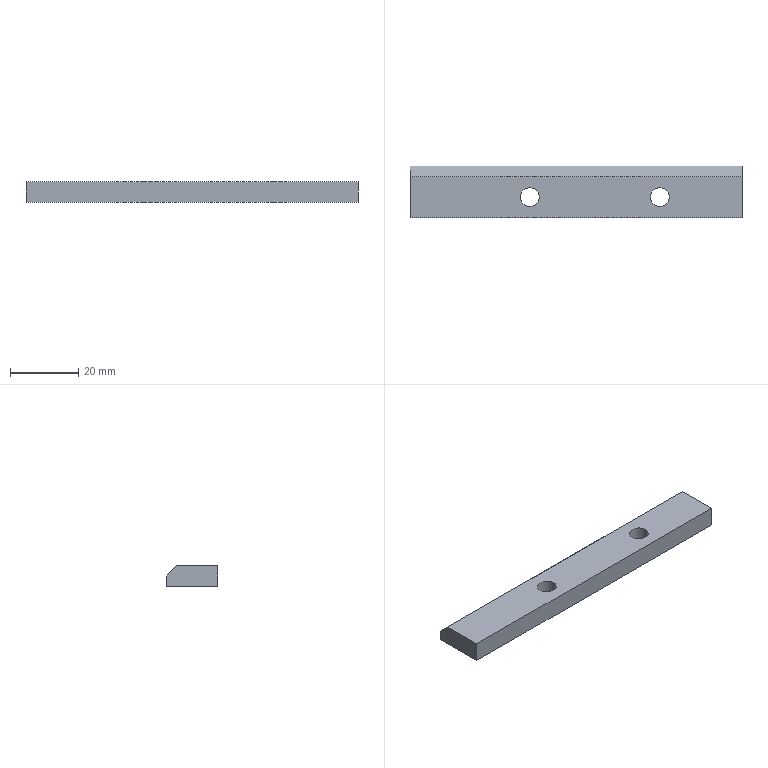Part | STEP file | cover plate 2 | 1 solid | 11 faces | box 97 x 15 x 6 mm | volume 8008 mm3 | plane 7 | cylinder 4 | commonest cylinder face diameters 5.5 x4
STEP:
#1=CARTESIAN_POINT('',(0.,0.,0.));
#2=DIRECTION('',(0.,0.,1.));
#3=DIRECTION('',(1.,0.,0.));
#4=AXIS2_PLACEMENT_3D('',#1,#2,#3);
#5=CARTESIAN_POINT('',(35.967,8.,0.));
#6=VERTEX_POINT('',#5);
#7=CARTESIAN_POINT('',(35.967,8.,6.));
#8=VERTEX_POINT('',#7);
#9=CARTESIAN_POINT('',(35.967,8.,6.));
#10=DIRECTION('',(0.,0.,1.));
#11=VECTOR('',#10,1.);
#12=LINE('',#9,#11);
#13=CARTESIAN_POINT('',(33.217,8.,6.));
#14=DIRECTION('',(0.,0.,1.));
#15=DIRECTION('',(1.,0.,0.));
#16=AXIS2_PLACEMENT_3D('',#13,#14,#15);
#17=CYLINDRICAL_SURFACE('',#16,2.75);
#18=CARTESIAN_POINT('',(6.283,0.));
#19=DIRECTION('',(0.,1.));
#20=VECTOR('',#19,1.);
#21=LINE('',#18,#20);
#22=(GEOMETRIC_REPRESENTATION_CONTEXT(2)PARAMETRIC_REPRESENTATION_CONTEXT()REPRESENTATION_CONTEXT('',''));
#23=DEFINITIONAL_REPRESENTATION('',(#21),#22);
#24=PCURVE('',#17,#23);
#25=CARTESIAN_POINT('',(33.217,8.,6.));
#26=DIRECTION('',(0.,0.,1.));
#27=DIRECTION('',(1.,0.,0.));
#28=AXIS2_PLACEMENT_3D('',#25,#26,#27);
#29=CYLINDRICAL_SURFACE('',#28,2.75);
#30=CARTESIAN_POINT('',(0.,0.));
#31=DIRECTION('',(0.,1.));
#32=VECTOR('',#31,1.);
#33=LINE('',#30,#32);
#34=(GEOMETRIC_REPRESENTATION_CONTEXT(2)PARAMETRIC_REPRESENTATION_CONTEXT()REPRESENTATION_CONTEXT('',''));
#35=DEFINITIONAL_REPRESENTATION('',(#33),#34);
#36=PCURVE('',#29,#35);
#37=SURFACE_CURVE('',#12,(#24,#36),.PCURVE_S1.);
#38=EDGE_CURVE('',#6,#8,#37,.T.);
#39=ORIENTED_EDGE('',*,*,#38,.T.);
#40=CARTESIAN_POINT('',(30.467,8.,6.));
#41=VERTEX_POINT('',#40);
#42=CARTESIAN_POINT('',(33.217,8.,6.));
#43=DIRECTION('',(0.,0.,1.));
#44=DIRECTION('',(1.,0.,0.));
#45=AXIS2_PLACEMENT_3D('',#42,#43,#44);
#46=CIRCLE('',#45,2.75);
#47=CARTESIAN_POINT('',(0.,0.));
#48=DIRECTION('',(1.,0.));
#49=VECTOR('',#48,1.);
#50=LINE('',#47,#49);
#51=(GEOMETRIC_REPRESENTATION_CONTEXT(2)PARAMETRIC_REPRESENTATION_CONTEXT()REPRESENTATION_CONTEXT('',''));
#52=DEFINITIONAL_REPRESENTATION('',(#50),#51);
#53=PCURVE('',#17,#52);
#54=CARTESIAN_POINT('',(40.217,2.,6.));
#55=DIRECTION('',(0.,0.,-1.));
#56=DIRECTION('',(-1.,0.,0.));
#57=AXIS2_PLACEMENT_3D('',#54,#55,#56);
#58=PLANE('',#57);
#59=CARTESIAN_POINT('',(4.25,6.));
#60=CARTESIAN_POINT('',(4.25,10.763));
#61=CARTESIAN_POINT('',(8.375,8.382));
#62=CARTESIAN_POINT('',(12.5,6.));
#63=CARTESIAN_POINT('',(8.375,3.618));
#64=CARTESIAN_POINT('',(4.25,1.237));
#65=CARTESIAN_POINT('',(4.25,6.));
#66=(BOUNDED_CURVE()B_SPLINE_CURVE(2,(#59,#60,#61,#62,#63,#64,#65),.UNSPECIFIED.,.T.,.F.)B_SPLINE_CURVE_WITH_KNOTS((1,2,2,2,2,1),(-2.094,0.,2.094,4.189,6.283,8.378),.UNSPECIFIED.)CURVE()GEOMETRIC_REPRESENTATION_ITEM()RATIONAL_B_SPLINE_CURVE((1.,0.5,1.,0.5,1.,0.5,1.))REPRESENTATION_ITEM(''));
#67=(GEOMETRIC_REPRESENTATION_CONTEXT(2)PARAMETRIC_REPRESENTATION_CONTEXT()REPRESENTATION_CONTEXT('',''));
#68=DEFINITIONAL_REPRESENTATION('',(#66),#67);
#69=PCURVE('',#58,#68);
#70=SURFACE_CURVE('',#46,(#53,#69),.PCURVE_S1.);
#71=EDGE_CURVE('',#41,#8,#70,.T.);
#72=ORIENTED_EDGE('',*,*,#71,.F.);
#73=CARTESIAN_POINT('',(30.467,8.,0.));
#74=VERTEX_POINT('',#73);
#75=CARTESIAN_POINT('',(30.467,8.,6.));
#76=DIRECTION('',(0.,0.,1.));
#77=VECTOR('',#76,1.);
#78=LINE('',#75,#77);
#79=CARTESIAN_POINT('',(3.142,0.));
#80=DIRECTION('',(0.,1.));
#81=VECTOR('',#80,1.);
#82=LINE('',#79,#81);
#83=(GEOMETRIC_REPRESENTATION_CONTEXT(2)PARAMETRIC_REPRESENTATION_CONTEXT()REPRESENTATION_CONTEXT('',''));
#84=DEFINITIONAL_REPRESENTATION('',(#82),#83);
#85=PCURVE('',#17,#84);
#86=CARTESIAN_POINT('',(3.142,0.));
#87=DIRECTION('',(0.,1.));
#88=VECTOR('',#87,1.);
#89=LINE('',#86,#88);
#90=(GEOMETRIC_REPRESENTATION_CONTEXT(2)PARAMETRIC_REPRESENTATION_CONTEXT()REPRESENTATION_CONTEXT('',''));
#91=DEFINITIONAL_REPRESENTATION('',(#89),#90);
#92=PCURVE('',#29,#91);
#93=SURFACE_CURVE('',#78,(#85,#92),.PCURVE_S1.);
#94=EDGE_CURVE('',#74,#41,#93,.T.);
#95=ORIENTED_EDGE('',*,*,#94,.F.);
#96=CARTESIAN_POINT('',(33.217,8.,0.));
#97=DIRECTION('',(0.,0.,-1.));
#98=DIRECTION('',(-1.,0.,0.));
#99=AXIS2_PLACEMENT_3D('',#96,#97,#98);
#100=CIRCLE('',#99,2.75);
#101=CARTESIAN_POINT('',(9.425,-6.));
#102=DIRECTION('',(-1.,0.));
#103=VECTOR('',#102,1.);
#104=LINE('',#101,#103);
#105=(GEOMETRIC_REPRESENTATION_CONTEXT(2)PARAMETRIC_REPRESENTATION_CONTEXT()REPRESENTATION_CONTEXT('',''));
#106=DEFINITIONAL_REPRESENTATION('',(#104),#105);
#107=PCURVE('',#17,#106);
#108=CARTESIAN_POINT('',(40.217,2.,0.));
#109=DIRECTION('',(0.,0.,-1.));
#110=DIRECTION('',(-1.,0.,0.));
#111=AXIS2_PLACEMENT_3D('',#108,#109,#110);
#112=PLANE('',#111);
#113=CARTESIAN_POINT('',(7.,6.));
#114=DIRECTION('',(1.,0.));
#115=AXIS2_PLACEMENT_2D('',#113,#114);
#116=CIRCLE('',#115,2.75);
#117=(GEOMETRIC_REPRESENTATION_CONTEXT(2)PARAMETRIC_REPRESENTATION_CONTEXT()REPRESENTATION_CONTEXT('',''));
#118=DEFINITIONAL_REPRESENTATION('',(#116),#117);
#119=PCURVE('',#112,#118);
#120=SURFACE_CURVE('',#100,(#107,#119),.PCURVE_S1.);
#121=EDGE_CURVE('',#6,#74,#120,.T.);
#122=ORIENTED_EDGE('',*,*,#121,.F.);
#123=EDGE_LOOP('',(#39,#72,#95,#122));
#124=FACE_BOUND('',#123,.F.);
#125=ADVANCED_FACE('',(#124),#17,.F.);
#126=CARTESIAN_POINT('',(-2.033,8.,0.));
#127=VERTEX_POINT('',#126);
#128=CARTESIAN_POINT('',(-2.033,8.,6.));
#129=VERTEX_POINT('',#128);
#130=CARTESIAN_POINT('',(-2.033,8.,6.));
#131=DIRECTION('',(0.,0.,1.));
#132=VECTOR('',#131,1.);
#133=LINE('',#130,#132);
#134=CARTESIAN_POINT('',(-4.783,8.,6.));
#135=DIRECTION('',(0.,0.,1.));
#136=DIRECTION('',(1.,0.,0.));
#137=AXIS2_PLACEMENT_3D('',#134,#135,#136);
#138=CYLINDRICAL_SURFACE('',#137,2.75);
#139=CARTESIAN_POINT('',(6.283,0.));
#140=DIRECTION('',(0.,1.));
#141=VECTOR('',#140,1.);
#142=LINE('',#139,#141);
#143=(GEOMETRIC_REPRESENTATION_CONTEXT(2)PARAMETRIC_REPRESENTATION_CONTEXT()REPRESENTATION_CONTEXT('',''));
#144=DEFINITIONAL_REPRESENTATION('',(#142),#143);
#145=PCURVE('',#138,#144);
#146=CARTESIAN_POINT('',(-4.783,8.,6.));
#147=DIRECTION('',(0.,0.,1.));
#148=DIRECTION('',(1.,0.,0.));
#149=AXIS2_PLACEMENT_3D('',#146,#147,#148);
#150=CYLINDRICAL_SURFACE('',#149,2.75);
#151=CARTESIAN_POINT('',(0.,0.));
#152=DIRECTION('',(0.,1.));
#153=VECTOR('',#152,1.);
#154=LINE('',#151,#153);
#155=(GEOMETRIC_REPRESENTATION_CONTEXT(2)PARAMETRIC_REPRESENTATION_CONTEXT()REPRESENTATION_CONTEXT('',''));
#156=DEFINITIONAL_REPRESENTATION('',(#154),#155);
#157=PCURVE('',#150,#156);
#158=SURFACE_CURVE('',#133,(#145,#157),.PCURVE_S1.);
#159=EDGE_CURVE('',#127,#129,#158,.T.);
#160=ORIENTED_EDGE('',*,*,#159,.T.);
#161=CARTESIAN_POINT('',(-7.533,8.,6.));
#162=VERTEX_POINT('',#161);
#163=CARTESIAN_POINT('',(-4.783,8.,6.));
#164=DIRECTION('',(0.,0.,1.));
#165=DIRECTION('',(1.,0.,0.));
#166=AXIS2_PLACEMENT_3D('',#163,#164,#165);
#167=CIRCLE('',#166,2.75);
#168=CARTESIAN_POINT('',(0.,0.));
#169=DIRECTION('',(1.,0.));
#170=VECTOR('',#169,1.);
#171=LINE('',#168,#170);
#172=(GEOMETRIC_REPRESENTATION_CONTEXT(2)PARAMETRIC_REPRESENTATION_CONTEXT()REPRESENTATION_CONTEXT('',''));
#173=DEFINITIONAL_REPRESENTATION('',(#171),#172);
#174=PCURVE('',#138,#173);
#175=CARTESIAN_POINT('',(42.25,6.));
#176=CARTESIAN_POINT('',(42.25,10.763));
#177=CARTESIAN_POINT('',(46.375,8.382));
#178=CARTESIAN_POINT('',(50.5,6.));
#179=CARTESIAN_POINT('',(46.375,3.618));
#180=CARTESIAN_POINT('',(42.25,1.237));
#181=CARTESIAN_POINT('',(42.25,6.));
#182=(BOUNDED_CURVE()B_SPLINE_CURVE(2,(#175,#176,#177,#178,#179,#180,#181),.UNSPECIFIED.,.T.,.F.)B_SPLINE_CURVE_WITH_KNOTS((1,2,2,2,2,1),(-2.094,0.,2.094,4.189,6.283,8.378),.UNSPECIFIED.)CURVE()GEOMETRIC_REPRESENTATION_ITEM()RATIONAL_B_SPLINE_CURVE((1.,0.5,1.,0.5,1.,0.5,1.))REPRESENTATION_ITEM(''));
#183=(GEOMETRIC_REPRESENTATION_CONTEXT(2)PARAMETRIC_REPRESENTATION_CONTEXT()REPRESENTATION_CONTEXT('',''));
#184=DEFINITIONAL_REPRESENTATION('',(#182),#183);
#185=PCURVE('',#58,#184);
#186=SURFACE_CURVE('',#167,(#174,#185),.PCURVE_S1.);
#187=EDGE_CURVE('',#162,#129,#186,.T.);
#188=ORIENTED_EDGE('',*,*,#187,.F.);
#189=CARTESIAN_POINT('',(-7.533,8.,0.));
#190=VERTEX_POINT('',#189);
#191=CARTESIAN_POINT('',(-7.533,8.,6.));
#192=DIRECTION('',(0.,0.,1.));
#193=VECTOR('',#192,1.);
#194=LINE('',#191,#193);
#195=CARTESIAN_POINT('',(3.142,0.));
#196=DIRECTION('',(0.,1.));
#197=VECTOR('',#196,1.);
#198=LINE('',#195,#197);
#199=(GEOMETRIC_REPRESENTATION_CONTEXT(2)PARAMETRIC_REPRESENTATION_CONTEXT()REPRESENTATION_CONTEXT('',''));
#200=DEFINITIONAL_REPRESENTATION('',(#198),#199);
#201=PCURVE('',#138,#200);
#202=CARTESIAN_POINT('',(3.142,0.));
#203=DIRECTION('',(0.,1.));
#204=VECTOR('',#203,1.);
#205=LINE('',#202,#204);
#206=(GEOMETRIC_REPRESENTATION_CONTEXT(2)PARAMETRIC_REPRESENTATION_CONTEXT()REPRESENTATION_CONTEXT('',''));
#207=DEFINITIONAL_REPRESENTATION('',(#205),#206);
#208=PCURVE('',#150,#207);
#209=SURFACE_CURVE('',#194,(#201,#208),.PCURVE_S1.);
#210=EDGE_CURVE('',#190,#162,#209,.T.);
#211=ORIENTED_EDGE('',*,*,#210,.F.);
#212=CARTESIAN_POINT('',(-4.783,8.,0.));
#213=DIRECTION('',(0.,0.,-1.));
#214=DIRECTION('',(-1.,0.,0.));
#215=AXIS2_PLACEMENT_3D('',#212,#213,#214);
#216=CIRCLE('',#215,2.75);
#217=CARTESIAN_POINT('',(9.425,-6.));
#218=DIRECTION('',(-1.,0.));
#219=VECTOR('',#218,1.);
#220=LINE('',#217,#219);
#221=(GEOMETRIC_REPRESENTATION_CONTEXT(2)PARAMETRIC_REPRESENTATION_CONTEXT()REPRESENTATION_CONTEXT('',''));
#222=DEFINITIONAL_REPRESENTATION('',(#220),#221);
#223=PCURVE('',#138,#222);
#224=CARTESIAN_POINT('',(45.,6.));
#225=DIRECTION('',(1.,0.));
#226=AXIS2_PLACEMENT_2D('',#224,#225);
#227=CIRCLE('',#226,2.75);
#228=(GEOMETRIC_REPRESENTATION_CONTEXT(2)PARAMETRIC_REPRESENTATION_CONTEXT()REPRESENTATION_CONTEXT('',''));
#229=DEFINITIONAL_REPRESENTATION('',(#227),#228);
#230=PCURVE('',#112,#229);
#231=SURFACE_CURVE('',#216,(#223,#230),.PCURVE_S1.);
#232=EDGE_CURVE('',#127,#190,#231,.T.);
#233=ORIENTED_EDGE('',*,*,#232,.F.);
#234=EDGE_LOOP('',(#160,#188,#211,#233));
#235=FACE_BOUND('',#234,.F.);
#236=ADVANCED_FACE('',(#235),#138,.F.);
#237=CARTESIAN_POINT('',(-39.783,2.,0.));
#238=VERTEX_POINT('',#237);
#239=CARTESIAN_POINT('',(57.217,2.,0.));
#240=VERTEX_POINT('',#239);
#241=CARTESIAN_POINT('',(-19.783,2.,0.));
#242=DIRECTION('',(1.,0.,0.));
#243=VECTOR('',#242,1.);
#244=LINE('',#241,#243);
#245=CARTESIAN_POINT('',(-19.783,2.,6.));
#246=DIRECTION('',(0.,1.,0.));
#247=DIRECTION('',(-1.,0.,0.));
#248=AXIS2_PLACEMENT_3D('',#245,#246,#247);
#249=PLANE('',#248);
#250=CARTESIAN_POINT('',(0.,-6.));
#251=DIRECTION('',(-1.,0.));
#252=VECTOR('',#251,1.);
#253=LINE('',#250,#252);
#254=(GEOMETRIC_REPRESENTATION_CONTEXT(2)PARAMETRIC_REPRESENTATION_CONTEXT()REPRESENTATION_CONTEXT('',''));
#255=DEFINITIONAL_REPRESENTATION('',(#253),#254);
#256=PCURVE('',#249,#255);
#257=CARTESIAN_POINT('',(60.,0.));
#258=DIRECTION('',(-1.,0.));
#259=VECTOR('',#258,1.);
#260=LINE('',#257,#259);
#261=(GEOMETRIC_REPRESENTATION_CONTEXT(2)PARAMETRIC_REPRESENTATION_CONTEXT()REPRESENTATION_CONTEXT('',''));
#262=DEFINITIONAL_REPRESENTATION('',(#260),#261);
#263=PCURVE('',#112,#262);
#264=SURFACE_CURVE('',#244,(#256,#263),.PCURVE_S1.);
#265=EDGE_CURVE('',#238,#240,#264,.T.);
#266=ORIENTED_EDGE('',*,*,#265,.T.);
#267=CARTESIAN_POINT('',(57.217,2.,6.));
#268=VERTEX_POINT('',#267);
#269=CARTESIAN_POINT('',(57.217,2.,6.));
#270=DIRECTION('',(0.,0.,-1.));
#271=VECTOR('',#270,1.);
#272=LINE('',#269,#271);
#273=CARTESIAN_POINT('',(-77.,0.));
#274=DIRECTION('',(0.,-1.));
#275=VECTOR('',#274,1.);
#276=LINE('',#273,#275);
#277=(GEOMETRIC_REPRESENTATION_CONTEXT(2)PARAMETRIC_REPRESENTATION_CONTEXT()REPRESENTATION_CONTEXT('',''));
#278=DEFINITIONAL_REPRESENTATION('',(#276),#277);
#279=PCURVE('',#249,#278);
#280=CARTESIAN_POINT('',(57.217,17.,0.));
#281=DIRECTION('',(1.,0.,0.));
#282=DIRECTION('',(0.,1.,0.));
#283=AXIS2_PLACEMENT_3D('',#280,#281,#282);
#284=PLANE('',#283);
#285=CARTESIAN_POINT('',(-15.,6.));
#286=DIRECTION('',(0.,-1.));
#287=VECTOR('',#286,1.);
#288=LINE('',#285,#287);
#289=(GEOMETRIC_REPRESENTATION_CONTEXT(2)PARAMETRIC_REPRESENTATION_CONTEXT()REPRESENTATION_CONTEXT('',''));
#290=DEFINITIONAL_REPRESENTATION('',(#288),#289);
#291=PCURVE('',#284,#290);
#292=SURFACE_CURVE('',#272,(#279,#291),.PCURVE_S1.);
#293=EDGE_CURVE('',#268,#240,#292,.T.);
#294=ORIENTED_EDGE('',*,*,#293,.F.);
#295=CARTESIAN_POINT('',(-39.783,2.,6.));
#296=VERTEX_POINT('',#295);
#297=CARTESIAN_POINT('',(-19.783,2.,6.));
#298=DIRECTION('',(1.,0.,0.));
#299=VECTOR('',#298,1.);
#300=LINE('',#297,#299);
#301=CARTESIAN_POINT('',(0.,0.));
#302=DIRECTION('',(-1.,0.));
#303=VECTOR('',#302,1.);
#304=LINE('',#301,#303);
#305=(GEOMETRIC_REPRESENTATION_CONTEXT(2)PARAMETRIC_REPRESENTATION_CONTEXT()REPRESENTATION_CONTEXT('',''));
#306=DEFINITIONAL_REPRESENTATION('',(#304),#305);
#307=PCURVE('',#249,#306);
#308=CARTESIAN_POINT('',(60.,0.));
#309=DIRECTION('',(-1.,0.));
#310=VECTOR('',#309,1.);
#311=LINE('',#308,#310);
#312=(GEOMETRIC_REPRESENTATION_CONTEXT(2)PARAMETRIC_REPRESENTATION_CONTEXT()REPRESENTATION_CONTEXT('',''));
#313=DEFINITIONAL_REPRESENTATION('',(#311),#312);
#314=PCURVE('',#58,#313);
#315=SURFACE_CURVE('',#300,(#307,#314),.PCURVE_S1.);
#316=EDGE_CURVE('',#296,#268,#315,.T.);
#317=ORIENTED_EDGE('',*,*,#316,.F.);
#318=CARTESIAN_POINT('',(-39.783,2.,0.));
#319=DIRECTION('',(0.,0.,1.));
#320=VECTOR('',#319,1.);
#321=LINE('',#318,#320);
#322=CARTESIAN_POINT('',(20.,-6.));
#323=DIRECTION('',(0.,1.));
#324=VECTOR('',#323,1.);
#325=LINE('',#322,#324);
#326=(GEOMETRIC_REPRESENTATION_CONTEXT(2)PARAMETRIC_REPRESENTATION_CONTEXT()REPRESENTATION_CONTEXT('',''));
#327=DEFINITIONAL_REPRESENTATION('',(#325),#326);
#328=PCURVE('',#249,#327);
#329=CARTESIAN_POINT('',(-39.783,2.,6.));
#330=DIRECTION('',(-1.,0.,0.));
#331=DIRECTION('',(0.,-1.,0.));
#332=AXIS2_PLACEMENT_3D('',#329,#330,#331);
#333=PLANE('',#332);
#334=CARTESIAN_POINT('',(0.,-6.));
#335=DIRECTION('',(0.,1.));
#336=VECTOR('',#335,1.);
#337=LINE('',#334,#336);
#338=(GEOMETRIC_REPRESENTATION_CONTEXT(2)PARAMETRIC_REPRESENTATION_CONTEXT()REPRESENTATION_CONTEXT('',''));
#339=DEFINITIONAL_REPRESENTATION('',(#337),#338);
#340=PCURVE('',#333,#339);
#341=SURFACE_CURVE('',#321,(#328,#340),.PCURVE_S1.);
#342=EDGE_CURVE('',#238,#296,#341,.T.);
#343=ORIENTED_EDGE('',*,*,#342,.F.);
#344=EDGE_LOOP('',(#266,#294,#317,#343));
#345=FACE_BOUND('',#344,.T.);
#346=ADVANCED_FACE('',(#345),#249,.F.);
#347=CARTESIAN_POINT('',(57.217,17.,0.));
#348=VERTEX_POINT('',#347);
#349=CARTESIAN_POINT('',(-39.783,17.,0.));
#350=VERTEX_POINT('',#349);
#351=CARTESIAN_POINT('',(-19.783,17.,0.));
#352=DIRECTION('',(-1.,0.,0.));
#353=VECTOR('',#352,1.);
#354=LINE('',#351,#353);
#355=CARTESIAN_POINT('',(-19.783,17.,6.));
#356=DIRECTION('',(0.,-1.,0.));
#357=DIRECTION('',(0.,0.,-1.));
#358=AXIS2_PLACEMENT_3D('',#355,#356,#357);
#359=PLANE('',#358);
#360=CARTESIAN_POINT('',(6.,0.));
#361=DIRECTION('',(0.,-1.));
#362=VECTOR('',#361,1.);
#363=LINE('',#360,#362);
#364=(GEOMETRIC_REPRESENTATION_CONTEXT(2)PARAMETRIC_REPRESENTATION_CONTEXT()REPRESENTATION_CONTEXT('',''));
#365=DEFINITIONAL_REPRESENTATION('',(#363),#364);
#366=PCURVE('',#359,#365);
#367=CARTESIAN_POINT('',(60.,15.));
#368=DIRECTION('',(1.,0.));
#369=VECTOR('',#368,1.);
#370=LINE('',#367,#369);
#371=(GEOMETRIC_REPRESENTATION_CONTEXT(2)PARAMETRIC_REPRESENTATION_CONTEXT()REPRESENTATION_CONTEXT('',''));
#372=DEFINITIONAL_REPRESENTATION('',(#370),#371);
#373=PCURVE('',#112,#372);
#374=SURFACE_CURVE('',#354,(#366,#373),.PCURVE_S1.);
#375=EDGE_CURVE('',#348,#350,#374,.T.);
#376=ORIENTED_EDGE('',*,*,#375,.T.);
#377=CARTESIAN_POINT('',(-39.783,17.,3.));
#378=VERTEX_POINT('',#377);
#379=CARTESIAN_POINT('',(-39.783,17.,3.));
#380=DIRECTION('',(0.,0.,-1.));
#381=VECTOR('',#380,1.);
#382=LINE('',#379,#381);
#383=CARTESIAN_POINT('',(3.,-20.));
#384=DIRECTION('',(1.,0.));
#385=VECTOR('',#384,1.);
#386=LINE('',#383,#385);
#387=(GEOMETRIC_REPRESENTATION_CONTEXT(2)PARAMETRIC_REPRESENTATION_CONTEXT()REPRESENTATION_CONTEXT('',''));
#388=DEFINITIONAL_REPRESENTATION('',(#386),#387);
#389=PCURVE('',#359,#388);
#390=CARTESIAN_POINT('',(-15.,-3.));
#391=DIRECTION('',(0.,-1.));
#392=VECTOR('',#391,1.);
#393=LINE('',#390,#392);
#394=(GEOMETRIC_REPRESENTATION_CONTEXT(2)PARAMETRIC_REPRESENTATION_CONTEXT()REPRESENTATION_CONTEXT('',''));
#395=DEFINITIONAL_REPRESENTATION('',(#393),#394);
#396=PCURVE('',#333,#395);
#397=SURFACE_CURVE('',#382,(#389,#396),.PCURVE_S1.);
#398=EDGE_CURVE('',#378,#350,#397,.T.);
#399=ORIENTED_EDGE('',*,*,#398,.F.);
#400=CARTESIAN_POINT('',(57.217,17.,3.));
#401=VERTEX_POINT('',#400);
#402=CARTESIAN_POINT('',(-19.783,17.,3.));
#403=DIRECTION('',(1.,0.,0.));
#404=VECTOR('',#403,1.);
#405=LINE('',#402,#404);
#406=CARTESIAN_POINT('',(3.,0.));
#407=DIRECTION('',(0.,1.));
#408=VECTOR('',#407,1.);
#409=LINE('',#406,#408);
#410=(GEOMETRIC_REPRESENTATION_CONTEXT(2)PARAMETRIC_REPRESENTATION_CONTEXT()REPRESENTATION_CONTEXT('',''));
#411=DEFINITIONAL_REPRESENTATION('',(#409),#410);
#412=PCURVE('',#359,#411);
#413=CARTESIAN_POINT('',(40.217,14.,6.));
#414=DIRECTION('',(0.,-0.7071,-0.7071));
#415=DIRECTION('',(0.,0.7071,-0.7071));
#416=AXIS2_PLACEMENT_3D('',#413,#414,#415);
#417=PLANE('',#416);
#418=CARTESIAN_POINT('',(4.243,-60.));
#419=DIRECTION('',(0.,1.));
#420=VECTOR('',#419,1.);
#421=LINE('',#418,#420);
#422=(GEOMETRIC_REPRESENTATION_CONTEXT(2)PARAMETRIC_REPRESENTATION_CONTEXT()REPRESENTATION_CONTEXT('',''));
#423=DEFINITIONAL_REPRESENTATION('',(#421),#422);
#424=PCURVE('',#417,#423);
#425=SURFACE_CURVE('',#405,(#412,#424),.PCURVE_S1.);
#426=EDGE_CURVE('',#378,#401,#425,.T.);
#427=ORIENTED_EDGE('',*,*,#426,.T.);
#428=CARTESIAN_POINT('',(57.217,17.,0.));
#429=DIRECTION('',(0.,0.,1.));
#430=VECTOR('',#429,1.);
#431=LINE('',#428,#430);
#432=CARTESIAN_POINT('',(6.,77.));
#433=DIRECTION('',(-1.,0.));
#434=VECTOR('',#433,1.);
#435=LINE('',#432,#434);
#436=(GEOMETRIC_REPRESENTATION_CONTEXT(2)PARAMETRIC_REPRESENTATION_CONTEXT()REPRESENTATION_CONTEXT('',''));
#437=DEFINITIONAL_REPRESENTATION('',(#435),#436);
#438=PCURVE('',#359,#437);
#439=CARTESIAN_POINT('',(0.,0.));
#440=DIRECTION('',(0.,1.));
#441=VECTOR('',#440,1.);
#442=LINE('',#439,#441);
#443=(GEOMETRIC_REPRESENTATION_CONTEXT(2)PARAMETRIC_REPRESENTATION_CONTEXT()REPRESENTATION_CONTEXT('',''));
#444=DEFINITIONAL_REPRESENTATION('',(#442),#443);
#445=PCURVE('',#284,#444);
#446=SURFACE_CURVE('',#431,(#438,#445),.PCURVE_S1.);
#447=EDGE_CURVE('',#348,#401,#446,.T.);
#448=ORIENTED_EDGE('',*,*,#447,.F.);
#449=EDGE_LOOP('',(#376,#399,#427,#448));
#450=FACE_BOUND('',#449,.T.);
#451=ADVANCED_FACE('',(#450),#359,.F.);
#452=CARTESIAN_POINT('',(33.217,8.,6.));
#453=DIRECTION('',(0.,0.,1.));
#454=DIRECTION('',(1.,0.,0.));
#455=AXIS2_PLACEMENT_3D('',#452,#453,#454);
#456=CIRCLE('',#455,2.75);
#457=CARTESIAN_POINT('',(4.25,6.));
#458=CARTESIAN_POINT('',(4.25,10.763));
#459=CARTESIAN_POINT('',(8.375,8.382));
#460=CARTESIAN_POINT('',(12.5,6.));
#461=CARTESIAN_POINT('',(8.375,3.618));
#462=CARTESIAN_POINT('',(4.25,1.237));
#463=CARTESIAN_POINT('',(4.25,6.));
#464=(BOUNDED_CURVE()B_SPLINE_CURVE(2,(#457,#458,#459,#460,#461,#462,#463),.UNSPECIFIED.,.T.,.F.)B_SPLINE_CURVE_WITH_KNOTS((1,2,2,2,2,1),(-2.094,0.,2.094,4.189,6.283,8.378),.UNSPECIFIED.)CURVE()GEOMETRIC_REPRESENTATION_ITEM()RATIONAL_B_SPLINE_CURVE((1.,0.5,1.,0.5,1.,0.5,1.))REPRESENTATION_ITEM(''));
#465=(GEOMETRIC_REPRESENTATION_CONTEXT(2)PARAMETRIC_REPRESENTATION_CONTEXT()REPRESENTATION_CONTEXT('',''));
#466=DEFINITIONAL_REPRESENTATION('',(#464),#465);
#467=PCURVE('',#58,#466);
#468=CARTESIAN_POINT('',(0.,0.));
#469=DIRECTION('',(1.,0.));
#470=VECTOR('',#469,1.);
#471=LINE('',#468,#470);
#472=(GEOMETRIC_REPRESENTATION_CONTEXT(2)PARAMETRIC_REPRESENTATION_CONTEXT()REPRESENTATION_CONTEXT('',''));
#473=DEFINITIONAL_REPRESENTATION('',(#471),#472);
#474=PCURVE('',#29,#473);
#475=SURFACE_CURVE('',#456,(#467,#474),.PCURVE_S1.);
#476=EDGE_CURVE('',#8,#41,#475,.T.);
#477=ORIENTED_EDGE('',*,*,#476,.F.);
#478=ORIENTED_EDGE('',*,*,#71,.F.);
#479=EDGE_LOOP('',(#477,#478));
#480=FACE_BOUND('',#479,.T.);
#481=CARTESIAN_POINT('',(-4.783,8.,6.));
#482=DIRECTION('',(0.,0.,1.));
#483=DIRECTION('',(1.,0.,0.));
#484=AXIS2_PLACEMENT_3D('',#481,#482,#483);
#485=CIRCLE('',#484,2.75);
#486=CARTESIAN_POINT('',(42.25,6.));
#487=CARTESIAN_POINT('',(42.25,10.763));
#488=CARTESIAN_POINT('',(46.375,8.382));
#489=CARTESIAN_POINT('',(50.5,6.));
#490=CARTESIAN_POINT('',(46.375,3.618));
#491=CARTESIAN_POINT('',(42.25,1.237));
#492=CARTESIAN_POINT('',(42.25,6.));
#493=(BOUNDED_CURVE()B_SPLINE_CURVE(2,(#486,#487,#488,#489,#490,#491,#492),.UNSPECIFIED.,.T.,.F.)B_SPLINE_CURVE_WITH_KNOTS((1,2,2,2,2,1),(-2.094,0.,2.094,4.189,6.283,8.378),.UNSPECIFIED.)CURVE()GEOMETRIC_REPRESENTATION_ITEM()RATIONAL_B_SPLINE_CURVE((1.,0.5,1.,0.5,1.,0.5,1.))REPRESENTATION_ITEM(''));
#494=(GEOMETRIC_REPRESENTATION_CONTEXT(2)PARAMETRIC_REPRESENTATION_CONTEXT()REPRESENTATION_CONTEXT('',''));
#495=DEFINITIONAL_REPRESENTATION('',(#493),#494);
#496=PCURVE('',#58,#495);
#497=CARTESIAN_POINT('',(0.,0.));
#498=DIRECTION('',(1.,0.));
#499=VECTOR('',#498,1.);
#500=LINE('',#497,#499);
#501=(GEOMETRIC_REPRESENTATION_CONTEXT(2)PARAMETRIC_REPRESENTATION_CONTEXT()REPRESENTATION_CONTEXT('',''));
#502=DEFINITIONAL_REPRESENTATION('',(#500),#501);
#503=PCURVE('',#150,#502);
#504=SURFACE_CURVE('',#485,(#496,#503),.PCURVE_S1.);
#505=EDGE_CURVE('',#129,#162,#504,.T.);
#506=ORIENTED_EDGE('',*,*,#505,.F.);
#507=ORIENTED_EDGE('',*,*,#187,.F.);
#508=EDGE_LOOP('',(#506,#507));
#509=FACE_BOUND('',#508,.T.);
#510=ORIENTED_EDGE('',*,*,#316,.T.);
#511=CARTESIAN_POINT('',(57.217,14.,6.));
#512=VERTEX_POINT('',#511);
#513=CARTESIAN_POINT('',(57.217,14.,6.));
#514=DIRECTION('',(0.,-1.,0.));
#515=VECTOR('',#514,1.);
#516=LINE('',#513,#515);
#517=CARTESIAN_POINT('',(-17.,12.));
#518=DIRECTION('',(0.,-1.));
#519=VECTOR('',#518,1.);
#520=LINE('',#517,#519);
#521=(GEOMETRIC_REPRESENTATION_CONTEXT(2)PARAMETRIC_REPRESENTATION_CONTEXT()REPRESENTATION_CONTEXT('',''));
#522=DEFINITIONAL_REPRESENTATION('',(#520),#521);
#523=PCURVE('',#58,#522);
#524=CARTESIAN_POINT('',(-3.,6.));
#525=DIRECTION('',(-1.,0.));
#526=VECTOR('',#525,1.);
#527=LINE('',#524,#526);
#528=(GEOMETRIC_REPRESENTATION_CONTEXT(2)PARAMETRIC_REPRESENTATION_CONTEXT()REPRESENTATION_CONTEXT('',''));
#529=DEFINITIONAL_REPRESENTATION('',(#527),#528);
#530=PCURVE('',#284,#529);
#531=SURFACE_CURVE('',#516,(#523,#530),.PCURVE_S1.);
#532=EDGE_CURVE('',#512,#268,#531,.T.);
#533=ORIENTED_EDGE('',*,*,#532,.F.);
#534=CARTESIAN_POINT('',(-39.783,14.,6.));
#535=VERTEX_POINT('',#534);
#536=CARTESIAN_POINT('',(40.217,14.,6.));
#537=DIRECTION('',(-1.,0.,0.));
#538=VECTOR('',#537,1.);
#539=LINE('',#536,#538);
#540=CARTESIAN_POINT('',(0.,12.));
#541=DIRECTION('',(1.,0.));
#542=VECTOR('',#541,1.);
#543=LINE('',#540,#542);
#544=(GEOMETRIC_REPRESENTATION_CONTEXT(2)PARAMETRIC_REPRESENTATION_CONTEXT()REPRESENTATION_CONTEXT('',''));
#545=DEFINITIONAL_REPRESENTATION('',(#543),#544);
#546=PCURVE('',#58,#545);
#547=CARTESIAN_POINT('',(0.,0.));
#548=DIRECTION('',(0.,-1.));
#549=VECTOR('',#548,1.);
#550=LINE('',#547,#549);
#551=(GEOMETRIC_REPRESENTATION_CONTEXT(2)PARAMETRIC_REPRESENTATION_CONTEXT()REPRESENTATION_CONTEXT('',''));
#552=DEFINITIONAL_REPRESENTATION('',(#550),#551);
#553=PCURVE('',#417,#552);
#554=SURFACE_CURVE('',#539,(#546,#553),.PCURVE_S1.);
#555=EDGE_CURVE('',#512,#535,#554,.T.);
#556=ORIENTED_EDGE('',*,*,#555,.T.);
#557=CARTESIAN_POINT('',(-39.783,2.,6.));
#558=DIRECTION('',(0.,1.,0.));
#559=VECTOR('',#558,1.);
#560=LINE('',#557,#559);
#561=CARTESIAN_POINT('',(80.,0.));
#562=DIRECTION('',(0.,1.));
#563=VECTOR('',#562,1.);
#564=LINE('',#561,#563);
#565=(GEOMETRIC_REPRESENTATION_CONTEXT(2)PARAMETRIC_REPRESENTATION_CONTEXT()REPRESENTATION_CONTEXT('',''));
#566=DEFINITIONAL_REPRESENTATION('',(#564),#565);
#567=PCURVE('',#58,#566);
#568=CARTESIAN_POINT('',(0.,0.));
#569=DIRECTION('',(-1.,0.));
#570=VECTOR('',#569,1.);
#571=LINE('',#568,#570);
#572=(GEOMETRIC_REPRESENTATION_CONTEXT(2)PARAMETRIC_REPRESENTATION_CONTEXT()REPRESENTATION_CONTEXT('',''));
#573=DEFINITIONAL_REPRESENTATION('',(#571),#572);
#574=PCURVE('',#333,#573);
#575=SURFACE_CURVE('',#560,(#567,#574),.PCURVE_S1.);
#576=EDGE_CURVE('',#296,#535,#575,.T.);
#577=ORIENTED_EDGE('',*,*,#576,.F.);
#578=EDGE_LOOP('',(#510,#533,#556,#577));
#579=FACE_BOUND('',#578,.T.);
#580=ADVANCED_FACE('',(#480,#509,#579),#58,.F.);
#581=ORIENTED_EDGE('',*,*,#121,.F.);
#582=CARTESIAN_POINT('',(33.217,8.,0.));
#583=DIRECTION('',(0.,0.,-1.));
#584=DIRECTION('',(-1.,0.,0.));
#585=AXIS2_PLACEMENT_3D('',#582,#583,#584);
#586=CIRCLE('',#585,2.75);
#587=CARTESIAN_POINT('',(7.,6.));
#588=DIRECTION('',(1.,0.));
#589=AXIS2_PLACEMENT_2D('',#587,#588);
#590=CIRCLE('',#589,2.75);
#591=(GEOMETRIC_REPRESENTATION_CONTEXT(2)PARAMETRIC_REPRESENTATION_CONTEXT()REPRESENTATION_CONTEXT('',''));
#592=DEFINITIONAL_REPRESENTATION('',(#590),#591);
#593=PCURVE('',#112,#592);
#594=CARTESIAN_POINT('',(3.142,-6.));
#595=DIRECTION('',(-1.,0.));
#596=VECTOR('',#595,1.);
#597=LINE('',#594,#596);
#598=(GEOMETRIC_REPRESENTATION_CONTEXT(2)PARAMETRIC_REPRESENTATION_CONTEXT()REPRESENTATION_CONTEXT('',''));
#599=DEFINITIONAL_REPRESENTATION('',(#597),#598);
#600=PCURVE('',#29,#599);
#601=SURFACE_CURVE('',#586,(#593,#600),.PCURVE_S1.);
#602=EDGE_CURVE('',#74,#6,#601,.T.);
#603=ORIENTED_EDGE('',*,*,#602,.F.);
#604=EDGE_LOOP('',(#581,#603));
#605=FACE_BOUND('',#604,.T.);
#606=ORIENTED_EDGE('',*,*,#232,.F.);
#607=CARTESIAN_POINT('',(-4.783,8.,0.));
#608=DIRECTION('',(0.,0.,-1.));
#609=DIRECTION('',(-1.,0.,0.));
#610=AXIS2_PLACEMENT_3D('',#607,#608,#609);
#611=CIRCLE('',#610,2.75);
#612=CARTESIAN_POINT('',(45.,6.));
#613=DIRECTION('',(1.,0.));
#614=AXIS2_PLACEMENT_2D('',#612,#613);
#615=CIRCLE('',#614,2.75);
#616=(GEOMETRIC_REPRESENTATION_CONTEXT(2)PARAMETRIC_REPRESENTATION_CONTEXT()REPRESENTATION_CONTEXT('',''));
#617=DEFINITIONAL_REPRESENTATION('',(#615),#616);
#618=PCURVE('',#112,#617);
#619=CARTESIAN_POINT('',(3.142,-6.));
#620=DIRECTION('',(-1.,0.));
#621=VECTOR('',#620,1.);
#622=LINE('',#619,#621);
#623=(GEOMETRIC_REPRESENTATION_CONTEXT(2)PARAMETRIC_REPRESENTATION_CONTEXT()REPRESENTATION_CONTEXT('',''));
#624=DEFINITIONAL_REPRESENTATION('',(#622),#623);
#625=PCURVE('',#150,#624);
#626=SURFACE_CURVE('',#611,(#618,#625),.PCURVE_S1.);
#627=EDGE_CURVE('',#190,#127,#626,.T.);
#628=ORIENTED_EDGE('',*,*,#627,.F.);
#629=EDGE_LOOP('',(#606,#628));
#630=FACE_BOUND('',#629,.T.);
#631=ORIENTED_EDGE('',*,*,#265,.F.);
#632=CARTESIAN_POINT('',(-39.783,17.,0.));
#633=DIRECTION('',(0.,-1.,0.));
#634=VECTOR('',#633,1.);
#635=LINE('',#632,#634);
#636=CARTESIAN_POINT('',(80.,15.));
#637=DIRECTION('',(0.,-1.));
#638=VECTOR('',#637,1.);
#639=LINE('',#636,#638);
#640=(GEOMETRIC_REPRESENTATION_CONTEXT(2)PARAMETRIC_REPRESENTATION_CONTEXT()REPRESENTATION_CONTEXT('',''));
#641=DEFINITIONAL_REPRESENTATION('',(#639),#640);
#642=PCURVE('',#112,#641);
#643=CARTESIAN_POINT('',(-15.,-6.));
#644=DIRECTION('',(1.,0.));
#645=VECTOR('',#644,1.);
#646=LINE('',#643,#645);
#647=(GEOMETRIC_REPRESENTATION_CONTEXT(2)PARAMETRIC_REPRESENTATION_CONTEXT()REPRESENTATION_CONTEXT('',''));
#648=DEFINITIONAL_REPRESENTATION('',(#646),#647);
#649=PCURVE('',#333,#648);
#650=SURFACE_CURVE('',#635,(#642,#649),.PCURVE_S1.);
#651=EDGE_CURVE('',#350,#238,#650,.T.);
#652=ORIENTED_EDGE('',*,*,#651,.F.);
#653=ORIENTED_EDGE('',*,*,#375,.F.);
#654=CARTESIAN_POINT('',(57.217,2.,0.));
#655=DIRECTION('',(0.,1.,0.));
#656=VECTOR('',#655,1.);
#657=LINE('',#654,#656);
#658=CARTESIAN_POINT('',(-17.,0.));
#659=DIRECTION('',(0.,1.));
#660=VECTOR('',#659,1.);
#661=LINE('',#658,#660);
#662=(GEOMETRIC_REPRESENTATION_CONTEXT(2)PARAMETRIC_REPRESENTATION_CONTEXT()REPRESENTATION_CONTEXT('',''));
#663=DEFINITIONAL_REPRESENTATION('',(#661),#662);
#664=PCURVE('',#112,#663);
#665=CARTESIAN_POINT('',(-15.,0.));
#666=DIRECTION('',(1.,0.));
#667=VECTOR('',#666,1.);
#668=LINE('',#665,#667);
#669=(GEOMETRIC_REPRESENTATION_CONTEXT(2)PARAMETRIC_REPRESENTATION_CONTEXT()REPRESENTATION_CONTEXT('',''));
#670=DEFINITIONAL_REPRESENTATION('',(#668),#669);
#671=PCURVE('',#284,#670);
#672=SURFACE_CURVE('',#657,(#664,#671),.PCURVE_S1.);
#673=EDGE_CURVE('',#240,#348,#672,.T.);
#674=ORIENTED_EDGE('',*,*,#673,.F.);
#675=EDGE_LOOP('',(#631,#652,#653,#674));
#676=FACE_BOUND('',#675,.T.);
#677=ADVANCED_FACE('',(#605,#630,#676),#112,.T.);
#678=ORIENTED_EDGE('',*,*,#505,.F.);
#679=ORIENTED_EDGE('',*,*,#159,.F.);
#680=ORIENTED_EDGE('',*,*,#627,.F.);
#681=ORIENTED_EDGE('',*,*,#210,.T.);
#682=EDGE_LOOP('',(#678,#679,#680,#681));
#683=FACE_BOUND('',#682,.F.);
#684=ADVANCED_FACE('',(#683),#150,.F.);
#685=ORIENTED_EDGE('',*,*,#476,.F.);
#686=ORIENTED_EDGE('',*,*,#38,.F.);
#687=ORIENTED_EDGE('',*,*,#602,.F.);
#688=ORIENTED_EDGE('',*,*,#94,.T.);
#689=EDGE_LOOP('',(#685,#686,#687,#688));
#690=FACE_BOUND('',#689,.F.);
#691=ADVANCED_FACE('',(#690),#29,.F.);
#692=ORIENTED_EDGE('',*,*,#555,.F.);
#693=CARTESIAN_POINT('',(57.217,17.,3.));
#694=DIRECTION('',(0.,-0.7071,0.7071));
#695=VECTOR('',#694,1.);
#696=LINE('',#693,#695);
#697=CARTESIAN_POINT('',(4.243,17.));
#698=DIRECTION('',(-1.,0.));
#699=VECTOR('',#698,1.);
#700=LINE('',#697,#699);
#701=(GEOMETRIC_REPRESENTATION_CONTEXT(2)PARAMETRIC_REPRESENTATION_CONTEXT()REPRESENTATION_CONTEXT('',''));
#702=DEFINITIONAL_REPRESENTATION('',(#700),#701);
#703=PCURVE('',#417,#702);
#704=CARTESIAN_POINT('',(0.,3.));
#705=DIRECTION('',(-0.7071,0.7071));
#706=VECTOR('',#705,1.);
#707=LINE('',#704,#706);
#708=(GEOMETRIC_REPRESENTATION_CONTEXT(2)PARAMETRIC_REPRESENTATION_CONTEXT()REPRESENTATION_CONTEXT('',''));
#709=DEFINITIONAL_REPRESENTATION('',(#707),#708);
#710=PCURVE('',#284,#709);
#711=SURFACE_CURVE('',#696,(#703,#710),.PCURVE_S1.);
#712=EDGE_CURVE('',#401,#512,#711,.T.);
#713=ORIENTED_EDGE('',*,*,#712,.F.);
#714=ORIENTED_EDGE('',*,*,#426,.F.);
#715=CARTESIAN_POINT('',(-39.783,14.,6.));
#716=DIRECTION('',(0.,0.7071,-0.7071));
#717=VECTOR('',#716,1.);
#718=LINE('',#715,#717);
#719=CARTESIAN_POINT('',(0.,-80.));
#720=DIRECTION('',(1.,0.));
#721=VECTOR('',#720,1.);
#722=LINE('',#719,#721);
#723=(GEOMETRIC_REPRESENTATION_CONTEXT(2)PARAMETRIC_REPRESENTATION_CONTEXT()REPRESENTATION_CONTEXT('',''));
#724=DEFINITIONAL_REPRESENTATION('',(#722),#723);
#725=PCURVE('',#417,#724);
#726=CARTESIAN_POINT('',(-12.,0.));
#727=DIRECTION('',(-0.7071,-0.7071));
#728=VECTOR('',#727,1.);
#729=LINE('',#726,#728);
#730=(GEOMETRIC_REPRESENTATION_CONTEXT(2)PARAMETRIC_REPRESENTATION_CONTEXT()REPRESENTATION_CONTEXT('',''));
#731=DEFINITIONAL_REPRESENTATION('',(#729),#730);
#732=PCURVE('',#333,#731);
#733=SURFACE_CURVE('',#718,(#725,#732),.PCURVE_S1.);
#734=EDGE_CURVE('',#535,#378,#733,.T.);
#735=ORIENTED_EDGE('',*,*,#734,.F.);
#736=EDGE_LOOP('',(#692,#713,#714,#735));
#737=FACE_BOUND('',#736,.T.);
#738=ADVANCED_FACE('',(#737),#417,.F.);
#739=ORIENTED_EDGE('',*,*,#673,.T.);
#740=ORIENTED_EDGE('',*,*,#447,.T.);
#741=ORIENTED_EDGE('',*,*,#712,.T.);
#742=ORIENTED_EDGE('',*,*,#532,.T.);
#743=ORIENTED_EDGE('',*,*,#293,.T.);
#744=EDGE_LOOP('',(#739,#740,#741,#742,#743));
#745=FACE_BOUND('',#744,.T.);
#746=ADVANCED_FACE('',(#745),#284,.T.);
#747=ORIENTED_EDGE('',*,*,#342,.T.);
#748=ORIENTED_EDGE('',*,*,#576,.T.);
#749=ORIENTED_EDGE('',*,*,#734,.T.);
#750=ORIENTED_EDGE('',*,*,#398,.T.);
#751=ORIENTED_EDGE('',*,*,#651,.T.);
#752=EDGE_LOOP('',(#747,#748,#749,#750,#751));
#753=FACE_BOUND('',#752,.T.);
#754=ADVANCED_FACE('',(#753),#333,.T.);
#755=CLOSED_SHELL('',(#125,#236,#346,#451,#580,#677,#684,#691,#738,#746,#754));
#756=MANIFOLD_SOLID_BREP('',#755);
#757=(LENGTH_UNIT()NAMED_UNIT(*)SI_UNIT(.MILLI.,.METRE.));
#758=UNCERTAINTY_MEASURE_WITH_UNIT(LENGTH_MEASURE(0.0000001),#757,'','');
#759=(NAMED_UNIT(*)PLANE_ANGLE_UNIT()SI_UNIT($,.RADIAN.));
#760=(NAMED_UNIT(*)SI_UNIT($,.STERADIAN.)SOLID_ANGLE_UNIT());
#761=(GEOMETRIC_REPRESENTATION_CONTEXT(3)GLOBAL_UNCERTAINTY_ASSIGNED_CONTEXT((#758))GLOBAL_UNIT_ASSIGNED_CONTEXT((#757,#759,#760))REPRESENTATION_CONTEXT('',''));
#762=ADVANCED_BREP_SHAPE_REPRESENTATION('',(#4,#756),#761);